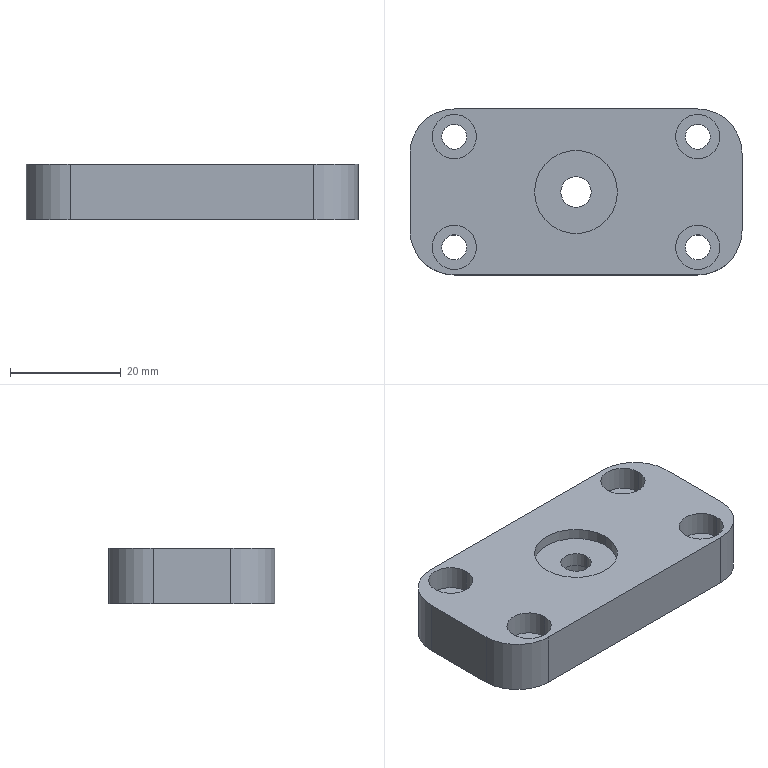Part | STEP file | 1 solid | 38 faces | box 60 x 30 x 10 mm | volume 15370 mm3 | cylinder 26 | plane 12 | commonest cylinder face diameters 4.5 x8 8 x8 16 x4 5.5 x2 10 x2 15 x2